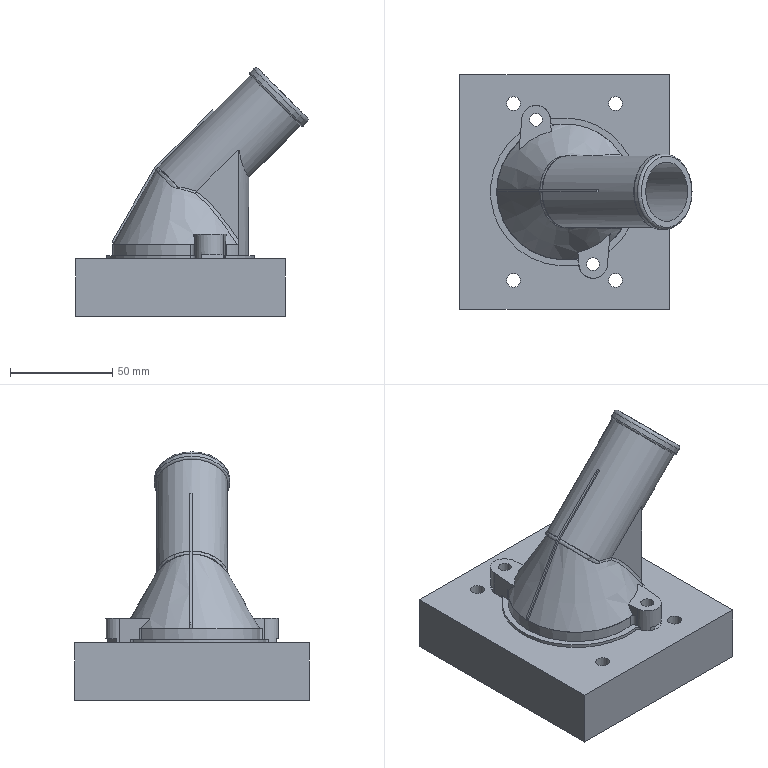CAM job | NX | 3-axis milling | part box 113.679 x 114.654 x 121.568 mm | stock box 400 x 400 x 380.568 mm
Tools:
number,name,description,diameter,corner_radius,flute_length,length,flutes
16,C-D16,Milling Tool-5 Parameters,16.0,0.0,40.0,75.0,21
12,C-D4,Milling Tool-5 Parameters,4.0,0.0,10.0,33.0,21
15,J-D10,Milling Tool-5 Parameters,10.0,0.0,30.0,65.0,21
5,J-D10R0.5,Milling Tool-5 Parameters,10.0,0.5,30.0,75.0,21
4,J-D4R0.5,Milling Tool-5 Parameters,4.0,0.5,10.0,25.0,21
6,J-D4R2,Milling Tool-Ball Mill,4.0,2.0,10.0,30.0,2
Operations:
program,operation,operation_type,tool,method,geometry_group,spindle_rpm,surface_speed,feed_per_tooth,feed_cut,feed_plunge,cut_length_mm,path_length_mm,cut_time_min,machine_time_min
A1,动态开粗,SurfaceContour,C-D16,END_MILL_MACRO,WP-1,7000.0,0.0,0.0,4000.0,100.0,60092.701,81086.725,13.033,15.133
A1,小孔开粗1,CylinderMilling,C-D16,END_MILL_MACRO,WP-1,7000.0,0.0,0.0,1000.0,100.0,5343.217,5556.894,5.343,5.365
A2,等高清角1,ZLevelMilling,C-D4,END_MILL_MACRO,WP-1,7000.0,301.0,0.1458,3000.0,50.0,1620.99,2968.084,0.5571,0.6918
A2,剩余铣粗,CavityMilling,C-D4,END_MILL_MACRO,WP-1,7000.0,100.0,0.1178,3500.0,100.0,6910.343,17177.502,1.974,3.001
A2,新底壁铣_1,VolumeBased25DMillingOperation,C-D4,END_MILL_MACRO,WP-1,8000.0,87.0,0.2143,700.0,250.0,86.309,281.363,0.0863,0.1058
A2,新底壁铣_1_COPY,VolumeBased25DMillingOperation,C-D4,END_MILL_MACRO,WP-1,8000.0,87.0,0.2143,700.0,250.0,86.443,279.497,0.0864,0.1057
A2,新底壁铣_1_COPY_COPY,VolumeBased25DMillingOperation,C-D4,END_MILL_MACRO,WP-1,8000.0,87.0,0.2143,700.0,250.0,186.696,381.365,0.1867,0.2062
A2,新底壁铣_1_COPY_COPY_COPY,VolumeBased25DMillingOperation,C-D4,END_MILL_MACRO,WP-1,8000.0,87.0,0.2143,700.0,250.0,187.285,402.052,0.1873,0.2088
A3,2D光侧面,FaceMilling,J-D10,END_MILL_MACRO,WP-1,7000.0,0.0,0.0,400.0,250.0,93.962,287.616,0.1002,0.1195
A3,2D光侧面_COPY,FaceMilling,J-D10,END_MILL_MACRO,WP-1,7000.0,0.0,0.0,400.0,250.0,94.01,285.664,0.1002,0.1194
A3,新底壁铣_2,VolumeBased25DMillingOperation,J-D10,END_MILL_MACRO,WP-1,7000.0,87.0,0.2143,400.0,250.0,112.881,417.017,0.1129,0.1433
A3,新底壁铣_2_COPY,VolumeBased25DMillingOperation,J-D10,END_MILL_MACRO,WP-1,7000.0,87.0,0.2143,400.0,250.0,249.918,908.678,0.2499,0.3158
A4,新底壁铣,VolumeBased25DMillingOperation,J-D10R0.5,END_MILL_MACRO,WP-1,7000.0,219.911,0.0048,700.0,100.0,351.867,499.594,0.5027,0.5174
A4,等高混合,ZLevelMilling,J-D10R0.5,END_MILL_MACRO,WP-1,8000.0,122.0,0.0044,2500.0,250.0,17372.078,17650.227,7.008,7.036
A4,等高顺铣,ZLevelMilling,J-D10R0.5,END_MILL_MACRO,WP-1,8000.0,122.0,0.0044,2500.0,250.0,4112.929,4264.017,1.656,1.671
A5,等高混合_1,ZLevelMilling,J-D4R0.5,END_MILL_MACRO,WP-1,8000.0,122.0,0.0044,2500.0,250.0,8959.592,10058.785,3.648,3.758
A6,精爬面,SurfaceContour,J-D4R2,END_MILL_MACRO,1-A,9000.0,0.0,0.0,3500.0,100.0,36346.602,41220.582,10.385,10.872
A6,精爬面_COPY,SurfaceContour,J-D4R2,END_MILL_MACRO,1-A,9000.0,0.0,0.0,3500.0,100.0,36778.238,42104.837,10.508,11.041
A7恢复工艺孔,小孔开粗1_1,CylinderMilling,J-D4R0.5,END_MILL_MACRO,WP-1,7000.0,0.0,0.0,1000.0,100.0,1136.34,1806.214,1.136,1.203